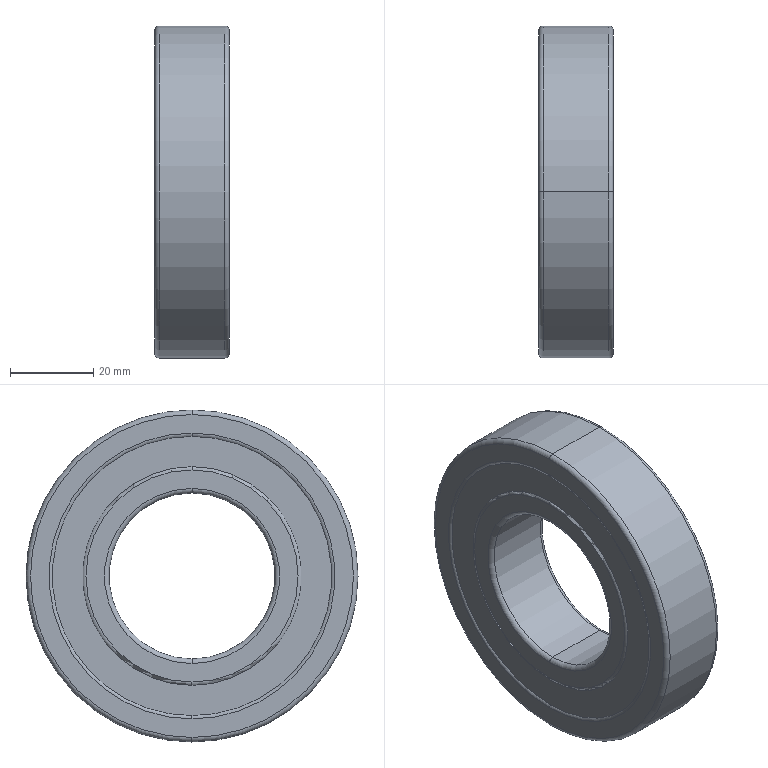Part | SolidWorks | features BaseBody 17 | 17 solids | 198 faces | box 18 x 80 x 80 mm | volume 52635 mm3 | cylinder 70 | sphere 64 | plane 38 | torus 26 | commonest cylinder face diameters 58 x29 62 x29 53.333 x4 66.667 x4 40 x2 80 x2